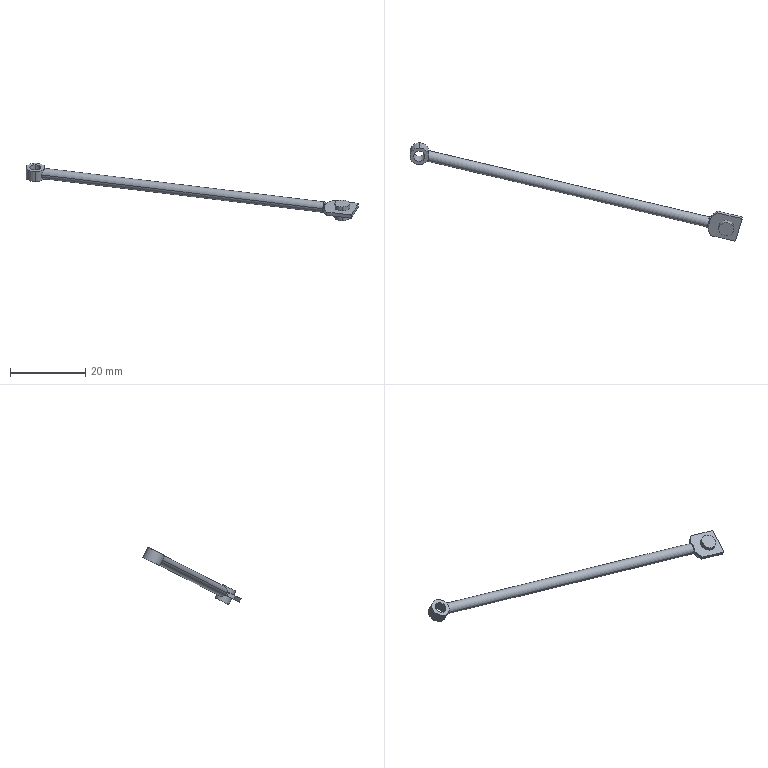Part | STEP file | Completa.sldasm-Part-142_Valor predeterminado | 1 solid | 29 faces | box 88.359 x 26.141 x 15.322 mm | volume 607.393 mm3 | cylinder 16 | plane 9 | spline 4 | commonest cylinder face diameters 9.6 x6 4 x4 2.8 x2 3 x2 5 x2